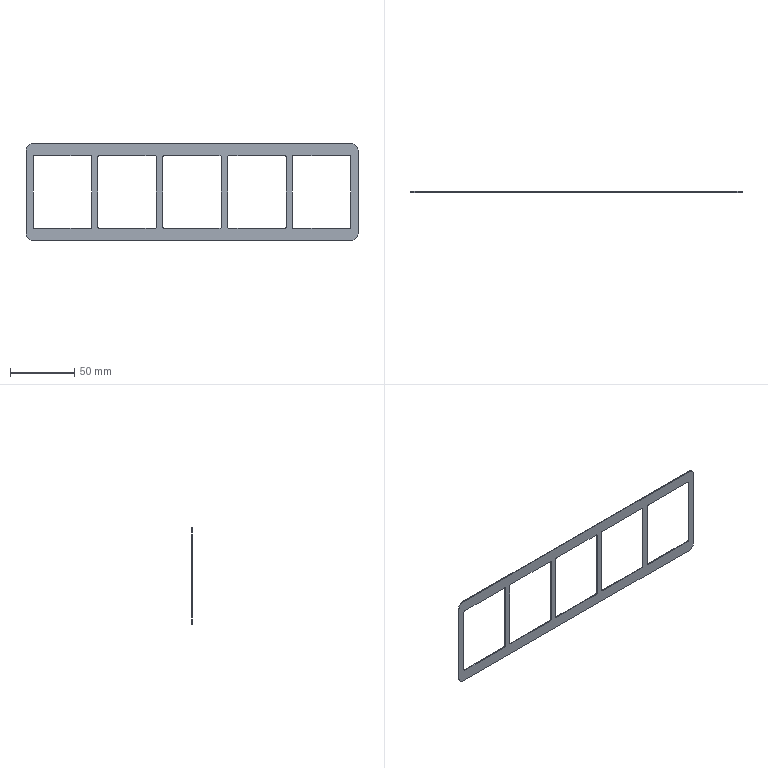Part | NX | features BREP 1 | 1 solid | 50 faces | box 258 x 0.7 x 75 mm | volume 4535 mm3 | plane 26 | cylinder 24 | commonest cylinder face diameters 2 x20 10 x4